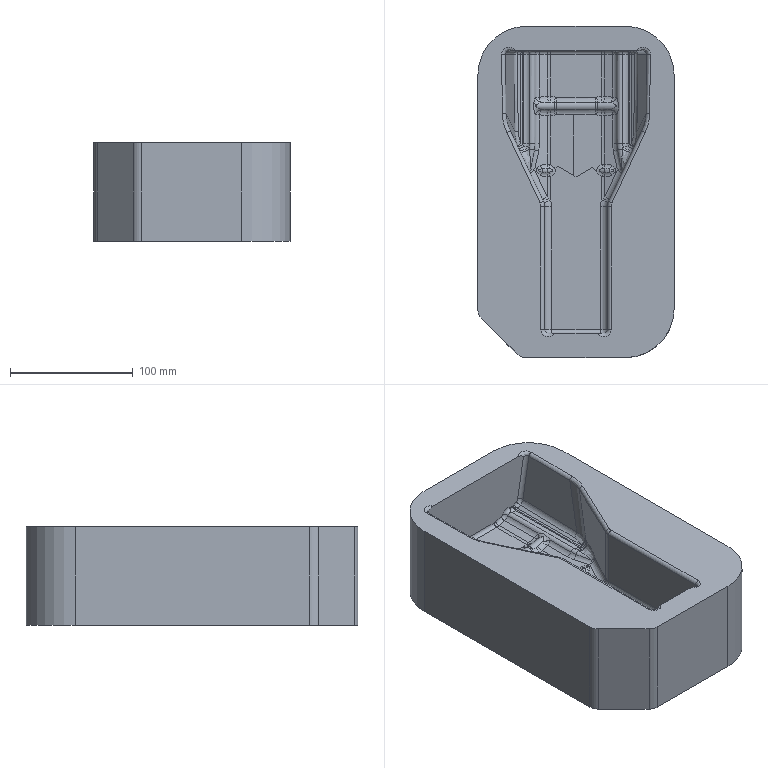NC program | NX | posted with a generic post | part box 160 x 270 x 80 mm
Lines 25870 to 26837 of 159324:
(ZLEVEL_PROFILE_1 , TOOL : D8)
N51726 M6
N51728 G54
N51730 G17 G0 G90 X4. Y107.025 S2800 M3
N51732 G43 Z10. H0
N51734 Z2.85
N51736 G94 G1 Z-0.15 F1500.
N51738 G3 X0. Y111.025 R4.
N51740 G1 X-50.377
N51742 G2 X-53.622 Y112.689 R4.032
N51744 G3 X-55.675 Y111.999 R1.155
N51746 G1 X-55.042 Y64.167
N51748 G3 X-51.869 Y50.51 R33.116
N51750 G1 X-24.871 Y-6.863
N51752 G2 X-23.737 Y-11.942 R11.936
N51754 G1 Y-112.025
N51756 G3 X-21.816 Y-112.655 R1.064
N51758 G2 X-18.589 Y-111.025 R4.042
N51760 G1 X18.593
N51762 G2 X21.816 Y-112.655 R4.041
N51764 G3 X23.737 Y-112.025 R1.064
N51766 G1 Y-11.942
N51768 G2 X24.871 Y-6.863 R11.936
N51770 G1 X51.869 Y50.51
N51772 G3 X55.042 Y64.167 R33.116
N51774 G1 X55.674 Y111.933
N51776 G3 X53.588 Y112.643 R1.159
N51778 G2 X50.377 Y111.025 R4.04
N51780 G1 X0.
N51782 Z-0.3
N51784 X50.847
N51786 G3 X53.898 Y112.439 R4.035
N51788 G2 X55.304 Y111.998 R0.794
N51790 G1 X54.671 Y64.172
N51792 G2 X51.533 Y50.668 R32.746
N51794 G1 X24.538 Y-6.7
N51796 G3 X23.366 Y-11.942 R12.307
N51798 G1 Y-112.025
N51800 G2 X22.149 Y-112.478 R0.693
N51802 G3 X19.061 Y-111.025 R4.037
N51804 G1 X-19.06
N51806 G3 X-22.14 Y-112.468 R4.038
N51808 G2 X-23.366 Y-112.025 R0.693
N51810 G1 Y-11.942
N51812 G3 X-24.538 Y-6.7 R12.307
N51814 G1 X-51.533 Y50.668
N51816 G2 X-54.671 Y64.172 R32.746
N51818 G1 X-55.304 Y112.017
N51820 G2 X-53.888 Y112.428 R0.792
N51822 G3 X-50.848 Y111.025 R4.028
N51824 G1 X0.
N51826 Z-0.45
N51828 X-51.214
N51830 G2 X-54.117 Y112.274 R4.055
N51832 G3 X-54.94 Y112.262 R0.563
N51834 X-55.032 Y112.021 R0.353
N51836 G1 X-54.399 Y64.175
N51838 G3 X-51.287 Y50.784 R32.473
N51840 G1 X-24.289 Y-6.588
N51842 G2 X-23.093 Y-11.942 R12.58
N51844 G1 Y-112.025
N51846 G3 X-22.371 Y-112.318 R0.42
N51848 G2 X-19.426 Y-111.025 R4.036
N51850 G1 X19.426
N51852 G2 X22.364 Y-112.31 R4.033
N51854 G3 X23.093 Y-112.025 R0.42
N51856 G1 Y-11.942
N51858 G2 X24.289 Y-6.588 R12.58
N51860 G1 X51.287 Y50.784
N51862 G3 X54.399 Y64.175 R32.473
N51864 G1 X55.031 Y111.948
N51866 G3 X54.165 Y112.303 R0.503
N51868 G2 X51.214 Y111.025 R4.158
N51870 G1 X0.
N51872 Z-0.599
N51874 X51.524
N51876 G3 X54.326 Y112.165 R4.081
N51878 G2 X54.812 Y112.006 R0.298
N51880 G1 X54.179 Y64.178
N51882 G2 X51.088 Y50.877 R32.253
N51884 G1 X24.094 Y-6.488
N51886 G3 X22.874 Y-11.942 R12.799
N51888 G1 Y-112.025
N51890 G2 X22.535 Y-112.17 R0.201
N51892 G3 X19.73 Y-111.025 R4.079
N51894 G1 X-19.73
N51896 G3 X-22.535 Y-112.17 R4.081
N51898 G2 X-22.874 Y-112.025 R0.201
N51900 G1 Y-11.942
N51902 G3 X-24.094 Y-6.488 R12.799
N51904 G1 X-51.088 Y50.877
N51906 G2 X-54.179 Y64.178 R32.253
N51908 G1 X-54.812 Y112.005
N51910 G2 X-54.328 Y112.165 R0.297
N51912 G3 X-51.523 Y111.025 R4.096
N51914 G1 X0.
N51916 Z-0.749
N51918 X-51.797
N51920 G2 X-54.42 Y112.002 R4.072
N51922 G3 X-54.627 Y112.002 R0.153
N51924 G1 X-53.995 Y64.181
N51926 G3 X-50.921 Y50.956 R32.069
N51928 G1 X-23.923 Y-6.418
N51930 G2 X-22.69 Y-11.942 R12.983
N51932 G1 Y-112.025
N51934 X-22.692 Y-112.04
N51936 X-22.679 Y-112.049
N51938 X-22.666 Y-112.04
N51940 G2 X-20. Y-111.025 R4.071
N51942 G1 X20.002
N51944 G2 X22.663 Y-112.038 R4.052
N51946 G1 X22.675 Y-112.05
N51948 X22.691 Y-112.042
N51950 X22.69 Y-112.025
N51952 Y-11.942
N51954 G2 X23.922 Y-6.42 R12.983
N51956 G1 X50.921 Y50.956
N51958 G3 X53.995 Y64.181 R32.069
N51960 G1 X54.627 Y112.001
N51962 G3 X54.43 Y112.01 R0.151
N51964 G2 X51.797 Y111.025 R4.088
N51966 G1 X0.
N51968 Z-0.899
N51970 X52.045
N51972 G3 X54.467 Y111.844 R4.019
N51974 G1 X53.837 Y64.215
N51976 G2 X50.778 Y51.023 R31.986
N51978 G1 X23.785 Y-6.339
N51980 G3 X22.531 Y-11.942 R13.142
N51982 G1 Y-111.744
N51984 G3 X20.246 Y-111.025 R4.013
N51986 G1 X-20.244
N51988 G3 X-22.531 Y-111.743 R4.039
N51990 G1 Y-11.942
N51992 G3 X-23.78 Y-6.351 R13.142
N51994 G1 X-50.778 Y51.023
N51996 G2 X-53.837 Y64.215 R31.986
N51998 G1 X-54.467 Y111.843
N52000 G3 X-52.046 Y111.025 R4.037
N52002 G1 X0.
N52004 Z-1.049
N52006 X-52.274
N52008 G2 X-54.327 Y111.595 R4.057
N52010 G1 X-53.7 Y64.184
N52012 G3 X-50.654 Y51.082 R31.774
N52014 G1 X-23.656 Y-6.293
N52016 G2 X-22.394 Y-11.942 R13.279
N52018 G1 Y-111.52
N52020 G2 X-20.469 Y-111.025 R4.055
N52022 G1 X20.471
N52024 G2 X22.394 Y-111.521 R4.028
N52026 G1 Y-11.942
N52028 G2 X23.661 Y-6.281 R13.279
N52030 G1 X50.654 Y51.082
N52032 G3 X53.7 Y64.184 R31.774
N52034 G1 X54.327 Y111.596
N52036 G2 X52.273 Y111.025 R4.033
N52038 G1 X0.
N52040 Z-1.199
N52042 X52.486
N52044 G3 X54.204 Y111.415 R4.012
N52046 G1 X53.579 Y64.186
N52048 G2 X50.545 Y51.133 R31.649
N52050 G1 X23.551 Y-6.233
N52052 G3 X22.274 Y-11.942 R13.399
N52054 G1 Y-111.357
N52056 G3 X20.68 Y-111.025 R4.089
N52058 G1 X-20.68
N52060 G3 X-22.274 Y-111.356 R4.093
N52062 G1 Y-11.942
N52064 G3 X-23.549 Y-6.236 R13.399
N52066 G1 X-50.545 Y51.133
N52068 G2 X-53.579 Y64.186 R31.654
N52070 G1 X-54.204 Y111.414
N52072 G3 X-52.486 Y111.025 R4.049
N52074 G1 X0.
N52076 Z-1.349
N52078 X-52.688
N52080 G2 X-54.097 Y111.283 R4.218
N52082 G1 X-53.479 Y64.606
N52084 X-53.474 Y64.206
N52086 X-53.465 Y63.807
N52088 X-53.454 Y63.407
N52090 X-53.437 Y63.007
N52092 G3 X-51.401 Y53.416 R31.376
N52094 X-50.374 Y51.018 R30.655
N52096 G1 X-23.455 Y-6.189
N52098 G2 X-22.168 Y-11.942 R13.505
N52100 G1 Y-111.24
N52102 G2 X-20.878 Y-111.025 R4.098
N52104 G1 X20.878
N52106 G2 X22.168 Y-111.239 R4.114
N52108 G1 Y-11.942
N52110 G2 X23.455 Y-6.189 R13.505
N52112 G1 X50.45 Y51.178
N52114 G3 X53.459 Y63.407 R31.802
N52116 G1 X53.465 Y63.807
N52118 X53.474 Y64.206
N52120 X53.479 Y64.606
N52122 X54.097 Y111.283
N52124 G2 X52.688 Y111.025 R4.141
N52126 G1 X0.
N52128 Z-1.499
N52130 X52.879
N52132 G3 X54.003 Y111.187 R4.064
N52134 G1 X53.381 Y64.189
N52136 X53.368 Y63.407
N52138 G2 X50.366 Y51.217 R31.754
N52140 G1 X23.37 Y-6.151
N52142 G3 X22.076 Y-11.942 R13.597
N52144 G1 Y-111.154
N52146 G3 X21.067 Y-111.025 R4.499
N52148 G1 X-21.066
N52150 G3 X-22.076 Y-111.155 R4.481
N52152 G1 Y-11.942
N52154 G3 X-23.37 Y-6.151 R13.597
N52156 G1 X-50.366 Y51.217
N52158 G2 X-53.144 Y60.775 R31.719
N52160 X-53.381 Y64.188 R30.529
N52162 G1 X-54.003 Y111.189
N52164 G3 X-52.88 Y111.025 R4.112
N52166 G1 X0.
N52168 Z-1.648
N52170 X-53.063
N52172 G2 X-53.921 Y111.121 R4.566
N52174 G1 X-53.3 Y64.19
N52176 G3 X-51.094 Y53.107 R31.351
N52178 X-50.293 Y51.252 R27.141
N52180 G1 X-23.299 Y-6.112
N52182 G2 X-21.995 Y-11.942 R13.678
N52184 G1 Y-111.097
N52186 G2 X-21.246 Y-111.025 R4.03
N52188 G1 X21.247
N52190 G2 X21.995 Y-111.097 R3.909
N52192 G1 Y-11.942
N52194 G2 X23.298 Y-6.115 R13.678
N52196 G1 X50.293 Y51.252
N52198 G3 X53.3 Y64.19 R31.374
N52200 G1 X53.921 Y111.119
N52202 G2 X53.063 Y111.025 R4.442
N52204 G1 X0.
N52206 Z-1.798
N52208 X53.239
N52210 G3 X53.85 Y111.07 R4.574
N52212 G1 X53.227 Y63.963
N52214 G2 X53.171 Y62.608 R24.528
N52216 X50.229 Y51.282 R31.696
N52218 G1 X23.234 Y-6.085
N52220 G3 X21.924 Y-11.942 R13.749
N52222 G1 Y-111.058
N52224 G3 X21.419 Y-111.025 R3.864
N52226 G1 X-21.419
N52228 G3 X-21.924 Y-111.058 R3.912
N52230 G1 Y-11.942
N52232 G3 X-23.23 Y-6.094 R13.749
N52234 G1 X-50.229 Y51.282
N52236 G2 X-51.892 Y55.627 R30.365
N52238 X-53.23 Y64.191 R30.959
N52240 G1 X-53.85 Y111.068
N52242 G3 X-53.239 Y111.025 R6.07
N52244 G1 X0.
N52246 Z-1.948
N52248 X-53.408
N52250 X-53.789 Y111.043
N52252 X-53.169 Y64.191
N52254 G3 X-50.174 Y51.308 R31.264
N52256 G1 X-23.175 Y-6.068
N52258 G2 X-21.863 Y-11.942 R13.81
N52260 G1 Y-111.028
N52262 X-21.587 Y-111.025
N52264 X21.863
N52266 Y-11.942
N52268 G2 X23.179 Y-6.06 R13.81
N52270 G1 X50.174 Y51.308
N52272 G3 X53.169 Y64.191 R31.272
N52274 G1 X53.789 Y111.043
N52276 X53.408 Y111.025
N52278 X0.
N52280 Z-2.098
N52282 X53.572
N52284 X53.737 Y111.029
N52286 X53.117 Y64.192
N52288 X53.081 Y63.007
N52290 G2 X51.018 Y53.416 R31.301
N52292 X50.115 Y51.303 R27.871
N52294 G1 X23.133 Y-6.035
N52296 G3 X21.812 Y-11.942 R13.861
N52298 G1 Y-111.025
N52300 X-21.75
N52302 X-21.812 Y-111.026
N52304 Y-11.942
N52306 G3 X-23.133 Y-6.035 R13.861
N52308 G1 X-50.127 Y51.33
N52310 G2 X-51.833 Y55.814 R30.884
N52312 X-53.117 Y64.192 R30.731
N52314 G1 X-53.737 Y111.029
N52316 X-53.572 Y111.025
N52318 X0.
N52320 Z-2.248
N52322 X-53.694
N52324 X-53.074 Y64.193
N52326 G3 X-51.892 Y56.17 R30.867
N52328 X-50.124 Y51.418 R31.407
N52330 G1 X-50.098 Y51.354
N52332 X-50.088 Y51.348
N52334 X-23.094 Y-6.017
N52336 G2 X-21.769 Y-11.942 R13.904
N52338 G1 Y-111.025
N52340 X21.769
N52342 Y-11.942
N52344 G2 X23.094 Y-6.017 R13.904
N52346 G1 X50.088 Y51.348
N52348 G3 X53.043 Y63.052 R31.415
N52350 X53.07 Y63.848 R19.549
N52352 G1 X53.694 Y111.025
N52354 X0.
N52356 Z-2.398
N52358 X53.659
N52360 X53.04 Y64.193
N52362 G2 X52.781 Y60.61 R29.881
N52364 X50.07 Y51.387 R31.668
N52366 G1 X50.057 Y51.363
N52368 X23.063 Y-6.002
N52370 G3 X21.734 Y-11.942 R13.939
N52372 G1 Y-111.025
N52374 X-21.734
N52376 Y-11.942
N52378 G3 X-23.063 Y-6.002 R13.939
N52380 G1 X-50.057 Y51.363
N52382 G2 X-53.033 Y63.807 R31.213
N52384 G1 X-53.04 Y63.834
N52386 G2 X-53.04 Y64.193 R1.717
N52388 G1 X-53.659 Y111.025
N52390 X0.
N52392 Z-2.548
N52394 X-53.632
N52396 X-53.012 Y64.174
N52398 G3 X-51.493 Y55.069 R30.796
N52400 X-50.032 Y51.374 R30.576
N52402 G1 X-23.039 Y-5.991
N52404 G2 X-21.707 Y-11.942 R13.966
N52406 G1 Y-111.025
N52408 X21.707
N52410 Y-11.942
N52412 G2 X23.039 Y-5.991 R13.966
N52414 G1 X50.032 Y51.374
N52416 G3 X52.976 Y63.007 R31.309
N52418 G1 X53.013 Y64.206
N52420 X53.632 Y111.025
N52422 X0.
N52424 Z-2.697
N52426 X53.606
N52428 X52.987 Y64.206
N52430 X52.952 Y63.007
N52432 G2 X50.033 Y51.418 R31.093
N52434 G1 X50.026 Y51.39
N52436 X50.015 Y51.382
N52438 X23.021 Y-5.983
N52440 G3 X21.688 Y-11.942 R13.985
N52442 G1 Y-111.025
N52444 X-21.688
N52446 Y-11.942
N52448 G3 X-23.022 Y-5.983 R13.985
N52450 G1 X-50.015 Y51.382
N52452 X-50.039 Y51.418
N52454 X-50.215 Y51.817
N52456 X-50.295 Y51.989
N52458 G2 X-52.986 Y64.118 R31.002
N52460 G1 X-53.606 Y111.025
N52462 X0.
N52464 Z-2.847
N52466 X-53.581
N52468 X-52.959 Y64.062
N52470 G3 X-50.005 Y51.387 R30.741
N52472 G1 X-23.011 Y-5.978
N52474 G2 X-21.677 Y-11.942 R13.996
N52476 G1 Y-111.025
N52478 X21.677
N52480 Y-11.942
N52482 G2 X23.011 Y-5.978 R13.996
N52484 G1 X50.005 Y51.387
N52486 G3 X52.961 Y64.206 R30.705
N52488 G1 X53.581 Y111.025
N52490 X0.
N52492 Z-2.997
N52494 X53.555
N52496 X52.936 Y64.206
N52498 G2 X50.015 Y51.418 R30.671
N52500 G1 X43.025 Y36.563
N52502 X23.005 Y-5.981
N52504 G3 X21.673 Y-11.932 R14.001
N52506 G1 Y-111.
N52508 Y-111.025
N52510 X-21.673
N52512 Y-110.997
N52514 Y-11.942
N52516 G3 X-23.011 Y-5.97 R14.014
N52518 G1 X-43.009 Y36.529
N52520 X-49.896 Y51.165
N52522 X-49.902 Y51.172
N52524 G2 X-52.933 Y64.006 R30.747
N52526 G1 X-53.555 Y111.025
N52528 X0.
N52530 Z-3.147
N52532 X-53.529
N52534 X-52.907 Y63.95
N52536 G3 X-49.976 Y51.334 R30.593
N52538 G1 X-23.008 Y-5.976
N52540 G2 X-21.673 Y-11.942 R14.
N52542 G1 Y-111.025
N52544 X21.673
N52546 Y-11.942
N52548 G2 X23.008 Y-5.976 R14.
N52550 G1 X49.976 Y51.334
N52552 G3 X52.91 Y64.206 R30.7
N52554 G1 X53.529 Y111.025
N52556 X0.
N52558 Z-3.297
N52560 X53.504
N52562 X52.885 Y64.206
N52564 G2 X49.949 Y51.278 R30.73
N52566 G1 X23.008 Y-5.976
N52568 G3 X21.673 Y-11.942 R14.
N52570 G1 Y-111.025
N52572 X-21.673
N52574 Y-11.942
N52576 G3 X-23.008 Y-5.976 R14.
N52578 G1 X-49.949 Y51.278
N52580 G2 X-52.88 Y63.894 R30.593
N52582 G1 X-53.504 Y111.025
N52584 X0.
N52586 Z-3.447
N52588 X-53.478
N52590 X-52.854 Y63.838
N52592 G3 X-49.923 Y51.222 R30.732
N52594 G1 X-23.008 Y-5.976
N52596 G2 X-21.673 Y-11.942 R14.
N52598 G1 Y-111.025
N52600 X21.673
N52602 Y-11.942
N52604 G2 X23.008 Y-5.976 R14.
N52606 G1 X49.934 Y51.245
N52608 G3 X52.855 Y63.921 R30.726
N52610 G1 X53.478 Y111.025
N52612 X0.
N52614 Z-3.597
N52616 X53.453
N52618 X52.828 Y63.807
N52620 G2 X49.897 Y51.166 R30.65
N52622 G1 X23.008 Y-5.976
N52624 G3 X21.673 Y-11.942 R14.
N52626 G1 Y-111.025
N52628 X-21.673
N52630 Y-11.942
N52632 G3 X-23.008 Y-5.976 R14.
N52634 G1 X-49.87 Y51.11
N52636 G2 X-52.828 Y63.807 R30.793
N52638 G1 X-53.453 Y111.025
N52640 X0.
N52642 Z-3.746
N52644 X-53.427
N52646 X-52.803 Y63.807
N52648 G3 X-49.87 Y51.11 R30.779
N52650 G1 X-23.008 Y-5.976
N52652 G2 X-21.673 Y-11.942 R14.
N52654 G1 Y-111.025
N52656 X21.673
N52658 Y-11.942
N52660 G2 X23.008 Y-5.976 R14.
N52662 G1 X49.897 Y51.166
N52664 G3 X52.803 Y63.807 R30.743
N52666 G1 X53.427 Y111.025
N52668 X0.
N52670 Z-3.896
N52672 X53.402
N52674 X52.775 Y63.67
N52676 G2 X52.657 Y61.409 R29.076
N52678 X49.87 Y51.11 R30.963
N52680 G1 X23.008 Y-5.976
N52682 G3 X21.673 Y-11.942 R14.
N52684 G1 Y-111.025
N52686 X-21.673
N52688 Y-11.942
N52690 G3 X-23.008 Y-5.976 R14.
N52692 G1 X-49.844 Y51.054
N52694 G2 X-52.777 Y63.807 R30.764
N52696 G1 X-53.402 Y111.025
N52698 X0.
N52700 Z-4.046
N52702 X-53.376
N52704 X-52.751 Y63.807
N52706 G3 X-49.818 Y50.998 R30.77
N52708 G1 X-23.008 Y-5.976
N52710 G2 X-21.673 Y-11.942 R14.
N52712 G1 Y-111.025
N52714 X21.673
N52716 Y-11.942
N52718 G2 X23.008 Y-5.976 R14.
N52720 G1 X49.844 Y51.054
N52722 G3 X51.924 Y57.013 R31.883
N52724 X52.751 Y63.807 R30.601
N52726 G1 X53.376 Y111.025
N52728 X0.
N52730 Z-4.196
N52732 X53.35
N52734 X52.726 Y63.807
N52736 G2 X51.367 Y55.014 R30.606
N52738 X49.818 Y50.998 R32.908
N52740 G1 X23.008 Y-5.976
N52742 G3 X21.673 Y-11.942 R14.
N52744 G1 Y-111.025
N52746 X-21.673
N52748 Y-11.942
N52750 G3 X-23.008 Y-5.976 R14.
N52752 G1 X-49.818 Y50.998
N52754 X-49.842 Y51.055
N52756 X-49.865 Y51.101
N52758 G2 X-52.726 Y63.807 R30.782
N52760 G1 X-53.35 Y111.025
N52762 X0.
N52764 Z-4.346
N52766 X-53.325
N52768 X-52.7 Y63.807
N52770 G3 X-49.864 Y51.102 R30.772
N52772 G1 X-49.841 Y51.055
N52774 X-49.792 Y50.942
N52776 X-23.008 Y-5.976
N52778 G2 X-21.673 Y-11.942 R14.
N52780 G1 Y-111.025
N52782 X21.673
N52784 Y-11.942
N52786 G2 X23.008 Y-5.976 R14.
N52788 G1 X49.791 Y50.942
N52790 G3 X50.578 Y52.783 R34.952
N52792 X52.697 Y63.555 R30.495
N52794 G1 X53.325 Y111.025
N52796 X0.
N52798 Z-4.496
N52800 X53.299
N52802 X52.671 Y63.496
N52804 G2 X50.557 Y52.741 R30.474
N52806 X49.765 Y50.886 R34.977
N52808 G1 X49.739 Y50.83
N52810 X23.008 Y-5.976
N52812 G3 X21.673 Y-11.942 R14.
N52814 G1 Y-111.025
N52816 X-21.673
N52818 Y-11.942
N52820 G3 X-23.008 Y-5.976 R14.
N52822 G1 X-49.739 Y50.83
N52824 X-49.978 Y51.361
N52826 G2 X-52.671 Y63.523 R30.638
N52828 G1 X-53.299 Y111.025
N52830 X0.
N52832 Z-4.646
N52834 X-53.274
N52836 X-52.645 Y63.468
N52838 G3 X-49.961 Y51.328 R30.634
N52840 G1 X-49.712 Y50.774
N52842 X-23.008 Y-5.976
N52844 G2 X-21.673 Y-11.942 R14.
N52846 G1 Y-111.025
N52848 X21.673
N52850 Y-11.942
N52852 G2 X23.008 Y-5.976 R14.
N52854 G1 X49.712 Y50.774
N52856 G3 X50.809 Y53.416 R34.765
N52858 X52.644 Y63.407 R30.706
N52860 G1 X52.649 Y63.807
N52862 X53.274 Y111.025
N52864 X0.
N52866 Z-4.795
N52868 X53.248
N52870 X52.618 Y63.407
N52872 G2 X50.803 Y53.416 R30.731
N52874 X49.686 Y50.719 R34.722
N52876 G1 X23.008 Y-5.976
N52878 G3 X21.673 Y-11.942 R14.
N52880 G1 Y-111.025
N52882 X-21.673
N52884 Y-11.942
N52886 G3 X-23.008 Y-5.976 R14.
N52888 G1 X-49.686 Y50.719
N52890 X-49.838 Y51.057
N52892 G2 X-52.618 Y63.407 R30.672
N52894 G1 X-53.248 Y111.025
N52896 X0.
N52898 Z-4.945
N52900 X-53.222
N52902 X-52.593 Y63.407
N52904 G3 X-49.808 Y50.992 R30.687
N52906 G1 X-49.66 Y50.663
N52908 X-23.008 Y-5.976
N52910 G2 X-21.673 Y-11.942 R14.
N52912 G1 Y-111.025
N52914 X21.673
N52916 Y-11.942
N52918 G2 X23.008 Y-5.976 R14.
N52920 G1 X49.66 Y50.663
N52922 G3 X51.199 Y54.615 R33.14
N52924 X52.593 Y63.407 R30.77
N52926 G1 X53.222 Y111.025
N52928 X0.
N52930 Z-5.095
N52932 X53.197
N52934 X52.567 Y63.407
N52936 G2 X51.19 Y54.615 R30.753
N52938 X49.633 Y50.607 R32.807
N52940 G1 X23.008 Y-5.976
N52942 G3 X21.673 Y-11.942 R14.
N52944 G1 Y-111.025
N52946 X-21.673
N52948 Y-11.942
N52950 G3 X-23.008 Y-5.976 R14.
N52952 G1 X-49.633 Y50.607
N52954 X-49.925 Y51.261
N52956 G2 X-52.566 Y63.295 R30.583
N52958 G1 X-53.197 Y111.025
N52960 X0.
N52962 Z-5.245
N52964 X-53.171
N52966 X-52.541 Y63.407
N52968 G3 X-49.755 Y50.88 R30.688
N52970 G1 X-49.733 Y50.833
N52972 X-49.607 Y50.551
N52974 X-23.008 Y-5.976
N52976 G2 X-21.673 Y-11.942 R14.
N52978 G1 Y-111.025
N52980 X21.673
N52982 Y-11.942
N52984 G2 X23.008 Y-5.976 R14.
N52986 G1 X49.633 Y50.607
N52988 G3 X51.502 Y55.732 R32.356
N52990 X52.541 Y63.407 R30.84
N52992 G1 X53.171 Y111.025
N52994 X0.
N52996 Z-5.395
N52998 X53.146
N53000 X52.516 Y63.407
N53002 G2 X51.29 Y55.014 R30.72
N53004 X49.607 Y50.551 R32.528
N53006 G1 X23.008 Y-5.976
N53008 G3 X21.673 Y-11.942 R14.
N53010 G1 Y-111.025
N53012 X-21.673
N53014 Y-11.942
N53016 G3 X-23.008 Y-5.976 R14.
N53018 G1 X-49.581 Y50.495
N53020 X-49.708 Y50.776
N53022 G2 X-52.516 Y63.407 R30.739
N53024 G1 X-53.146 Y111.025
N53026 X0.
N53028 Z-5.545
N53030 X-53.12
N53032 X-52.487 Y63.128
N53034 G3 X-49.73 Y50.834 R30.595
N53036 G1 X-49.706 Y50.777
N53038 X-49.678 Y50.711
N53040 X-49.554 Y50.439
N53042 X-23.008 Y-5.976
N53044 G2 X-21.673 Y-11.942 R14.
N53046 G1 Y-111.025
N53048 X21.673
N53050 Y-11.942
N53052 G2 X23.008 Y-5.976 R14.
N53054 G1 X49.581 Y50.495
N53056 G3 X50.907 Y53.815 R34.074
N53058 X52.486 Y63.069 R30.738
N53060 G1 X52.49 Y63.407
N53062 X53.12 Y111.025
N53064 X0.
N53066 Z-5.695
N53068 X53.095
N53070 X52.465 Y63.407
N53072 X52.459 Y63.013
N53074 G2 X50.704 Y53.248 R30.686
N53076 X49.554 Y50.439 R35.133
N53078 G1 X23.008 Y-5.976
N53080 G3 X21.673 Y-11.942 R14.
N53082 G1 Y-111.025
N53084 X-21.673
N53086 Y-11.942
N53088 G3 X-23.008 Y-5.976 R14.
N53090 G1 X-49.528 Y50.383
N53092 X-49.788 Y50.963
N53094 G2 X-52.46 Y63.075 R30.623
N53096 G1 X-53.095 Y111.025
N53098 X0.
N53100 Z-5.844
N53102 X-53.069
N53104 X-52.434 Y63.007
N53106 G3 X-49.704 Y50.778 R30.633
N53108 G1 X-49.502 Y50.327
N53110 X-23.008 Y-5.976
N53112 G2 X-21.673 Y-11.942 R14.
N53114 G1 Y-111.025
N53116 X21.673
N53118 Y-11.942
N53120 G2 X23.008 Y-5.976 R14.
N53122 G1 X49.502 Y50.327
N53124 G3 X50.305 Y52.192 R40.5
N53126 X52.434 Y63.007 R30.743
N53128 G1 X53.069 Y111.025
N53130 X0.
N53132 Z-5.994
N53134 X53.043
N53136 X52.408 Y63.007
N53138 G2 X50.608 Y53.016 R30.711
N53140 X49.475 Y50.271 R35.078
N53142 G1 X23.008 Y-5.976
N53144 G3 X21.673 Y-11.942 R14.
N53146 G1 Y-111.025
N53148 X-21.673
N53150 Y-11.942
N53152 G3 X-23.008 Y-5.976 R14.
N53154 G1 X-49.475 Y50.271
N53156 X-49.674 Y50.713
N53158 G2 X-52.408 Y63.007 R30.666
N53160 G1 X-53.043 Y111.025
N53162 X0.
N53164 Z-6.144
N53166 X-53.018
N53168 X-52.383 Y63.007
N53170 G3 X-49.626 Y50.61 R30.644
N53172 G1 X-49.449 Y50.215
N53174 X-23.008 Y-5.976
N53176 G2 X-21.673 Y-11.942 R14.
N53178 G1 Y-111.025
N53180 X21.673
N53182 Y-11.942
N53184 G2 X23.008 Y-5.976 R14.
N53186 G1 X49.449 Y50.215
N53188 G3 X50.603 Y53.016 R35.17
N53190 X52.383 Y63.007 R30.729
N53192 G1 X53.018 Y111.025
N53194 X0.
N53196 Z-6.294
N53198 X52.992
N53200 X52.357 Y63.007
N53202 G2 X50.595 Y53.016 R30.682
N53204 X49.449 Y50.215 R35.08
N53206 G1 X23.008 Y-5.976
N53208 G3 X21.673 Y-11.942 R14.
N53210 G1 Y-111.025
N53212 X-21.673
N53214 Y-11.942
N53216 G3 X-23.008 Y-5.976 R14.
N53218 G1 X-49.449 Y50.215
N53220 X-49.747 Y50.889
N53222 G2 X-52.355 Y62.848 R30.586
N53224 G1 X-52.992 Y111.025
N53226 X0.
N53228 Z-6.444
N53230 X-52.967
N53232 X-52.329 Y62.783
N53234 G3 X-49.748 Y50.895 R30.533
N53236 G1 X-49.523 Y50.385
N53238 X-49.397 Y50.103
N53240 X-23.008 Y-5.976
N53242 G2 X-21.673 Y-11.942 R14.
N53244 G1 Y-111.025
N53246 X21.673
N53248 Y-11.942
N53250 G2 X23.008 Y-5.976 R14.
N53252 G1 X49.423 Y50.159
N53254 G3 X50.725 Y53.416 R33.845
N53256 X52.332 Y63.007 R30.648
N53258 G1 X52.967 Y111.025
N53260 X0.
N53262 Z-6.594
N53264 X52.941
N53266 X52.306 Y63.007
N53268 X52.302 Y62.676
N53270 G2 X50.718 Y53.416 R30.656
N53272 X49.397 Y50.103 R33.528
N53274 G1 X23.008 Y-5.976
N53276 G3 X21.673 Y-11.942 R14.
N53278 G1 Y-111.025
N53280 X-21.673
N53282 Y-11.942
N53284 G3 X-23.008 Y-5.976 R14.
N53286 G1 X-49.37 Y50.047
N53288 X-49.423 Y50.159
N53290 X-49.706 Y50.8
N53292 G2 X-52.302 Y62.732 R30.571
N53294 G1 X-52.941 Y111.025
N53296 X0.
N53298 Z-6.744
N53300 X-52.915
N53302 X-52.276 Y62.693
N53304 G3 X-49.521 Y50.386 R30.684
N53306 G1 X-49.497 Y50.325
N53308 X-49.344 Y49.991
N53310 X-23.008 Y-5.976
N53312 G2 X-21.673 Y-11.942 R14.
N53314 G1 Y-111.025
N53316 X21.673
N53318 Y-11.942
N53320 G2 X23.008 Y-5.976 R14.
N53322 G1 X49.37 Y50.047
N53324 G3 X51.103 Y54.684 R32.535
N53326 X52.275 Y62.621 R30.716
N53328 G1 X52.28 Y63.007
N53330 X52.915 Y111.025
N53332 X0.
N53334 Z-6.893
N53336 X52.89
N53338 X52.249 Y62.608
N53340 G2 X51.103 Y54.721 R30.735
N53342 X49.344 Y49.991 R32.194
N53344 G1 X23.008 Y-5.976
N53346 G3 X21.673 Y-11.942 R14.
N53348 G1 Y-111.025
N53350 X-21.673
N53352 Y-11.942
N53354 G3 X-23.008 Y-5.976 R14.
N53356 G1 X-49.318 Y49.935
N53358 X-49.497 Y50.327
N53360 X-49.52 Y50.386
N53362 G2 X-52.249 Y62.608 R30.689
N53364 G1 X-52.89 Y111.025
N53366 X0.
N53368 Z-7.043
N53370 X-52.864
N53372 X-52.224 Y62.58
N53374 G3 X-49.529 Y50.409 R30.671
N53376 G1 X-49.291 Y49.879
N53378 X-23.008 Y-5.976
N53380 G2 X-21.673 Y-11.942 R14.
N53382 G1 Y-111.025
N53384 X21.673
N53386 Y-11.942
N53388 G2 X23.008 Y-5.976 R14.
N53390 G1 X49.291 Y49.879
N53392 X49.317 Y49.935
N53394 G3 X51.278 Y55.414 R32.045
N53396 X52.224 Y62.608 R30.768
N53398 G1 X52.864 Y111.025
N53400 X0.
N53402 Z-7.193
N53404 X52.839
N53406 X52.198 Y62.608
N53408 G2 X50.815 Y53.815 R30.756
N53410 X49.291 Y49.879 R32.87
N53412 G1 X23.008 Y-5.976
N53414 G3 X21.673 Y-11.942 R14.
N53416 G1 Y-111.025
N53418 X-21.673
N53420 Y-11.942
N53422 G3 X-23.008 Y-5.976 R14.
N53424 G1 X-49.265 Y49.824
N53426 X-49.412 Y50.152
N53428 G2 X-52.198 Y62.608 R30.707
N53430 G1 X-52.839 Y111.025
N53432 X0.
N53434 Z-7.343
N53436 X-52.813
N53438 X-52.171 Y62.466
N53440 G3 X-49.475 Y50.294 R30.663
N53442 G1 X-49.239 Y49.768
N53444 X-23.008 Y-5.976
N53446 G2 X-21.673 Y-11.942 R14.
N53448 G1 Y-111.025
N53450 X21.673
N53452 Y-11.942
N53454 G2 X23.008 Y-5.976 R14.
N53456 G1 X49.239 Y49.768
N53458 G3 X50.807 Y53.815 R32.671
N53460 X52.173 Y62.608 R30.792
N53462 G1 X52.813 Y111.025
N53464 X0.
N53466 Z-7.493
N53468 X52.788
N53470 X52.147 Y62.608
N53472 G2 X50.917 Y54.215 R30.786
N53474 X49.212 Y49.712 R32.355
N53476 G1 X23.008 Y-5.976
N53478 G3 X21.673 Y-11.942 R14.
N53480 G1 Y-111.025
N53482 X-21.673
N53484 Y-11.942
N53486 G3 X-23.008 Y-5.976 R14.
N53488 G1 X-49.212 Y49.712
N53490 X-49.425 Y50.182
N53492 G2 X-52.145 Y62.415 R30.699
N53494 G1 X-52.788 Y111.025
N53496 X0.
N53498 Z-7.643
N53500 X-52.762
N53502 X-52.118 Y62.355
N53504 G3 X-49.421 Y50.179 R30.671
N53506 G1 X-49.186 Y49.656
N53508 X-23.008 Y-5.976
N53510 G2 X-21.673 Y-11.942 R14.
N53512 G1 Y-111.025
N53514 X21.673
N53516 Y-11.942
N53518 G2 X23.008 Y-5.976 R14.
N53520 G1 X49.212 Y49.712
N53522 G3 X51.103 Y54.923 R32.233
N53524 X52.122 Y62.608 R30.813
N53526 G1 X52.762 Y111.025
N53528 X0.
N53530 Z-7.793
N53532 X52.736
N53534 X52.096 Y62.608
N53536 X52.091 Y62.23
N53538 G2 X50.387 Y52.617 R30.669
N53540 X49.186 Y49.656 R33.882
N53542 G1 X23.008 Y-5.976
N53544 G3 X21.673 Y-11.942 R14.
N53546 G1 Y-111.025
N53548 X-21.673
N53550 Y-11.942
N53552 G3 X-23.008 Y-5.976 R14.
N53554 G1 X-49.16 Y49.6
N53556 X-49.375 Y50.076
N53558 G2 X-52.092 Y62.303 R30.697
N53560 G1 X-52.736 Y111.025
N53562 X0.
N53564 Z-7.942
N53566 X-52.711
N53568 X-52.065 Y62.208
N53570 G3 X-49.286 Y49.882 R30.682
N53572 G1 X-49.281 Y49.873
N53574 X-49.16 Y49.6
N53576 X-23.008 Y-5.976
N53578 G2 X-21.673 Y-11.942 R14.
N53580 G1 Y-111.025
N53582 X21.673
N53584 Y-11.942
N53586 G2 X23.008 Y-5.976 R14.
N53588 G1 X49.133 Y49.544
N53590 X49.159 Y49.6
N53592 G3 X49.938 Y51.418 R37.202
N53594 X52.065 Y62.208 R30.728
N53596 G1 X52.711 Y111.025
N53598 X0.
N53600 Z-8.092
N53602 X52.685
N53604 X52.04 Y62.208
N53606 G2 X49.934 Y51.418 R30.719
N53608 X49.107 Y49.488 R36.205
N53610 G1 X23.008 Y-5.976
N53612 G3 X21.673 Y-11.942 R14.
N53614 G1 Y-111.025
N53616 X-21.673
N53618 Y-11.942
N53620 G3 X-23.008 Y-5.976 R14.
N53622 G1 X-49.107 Y49.488
N53624 X-49.234 Y49.77
N53626 G2 X-52.04 Y62.208 R30.715
N53628 G1 X-52.685 Y111.025
N53630 X0.
N53632 Z-8.242
N53634 X-52.66
N53636 X-52.014 Y62.208
N53638 G3 X-49.232 Y49.77 R30.69
N53640 G1 X-49.081 Y49.432
N53642 X-23.008 Y-5.976
N53644 G2 X-21.673 Y-11.942 R14.
N53646 G1 Y-111.025
N53648 X21.673
N53650 Y-11.942
N53652 G2 X23.008 Y-5.976 R14.
N53654 G1 X49.081 Y49.432